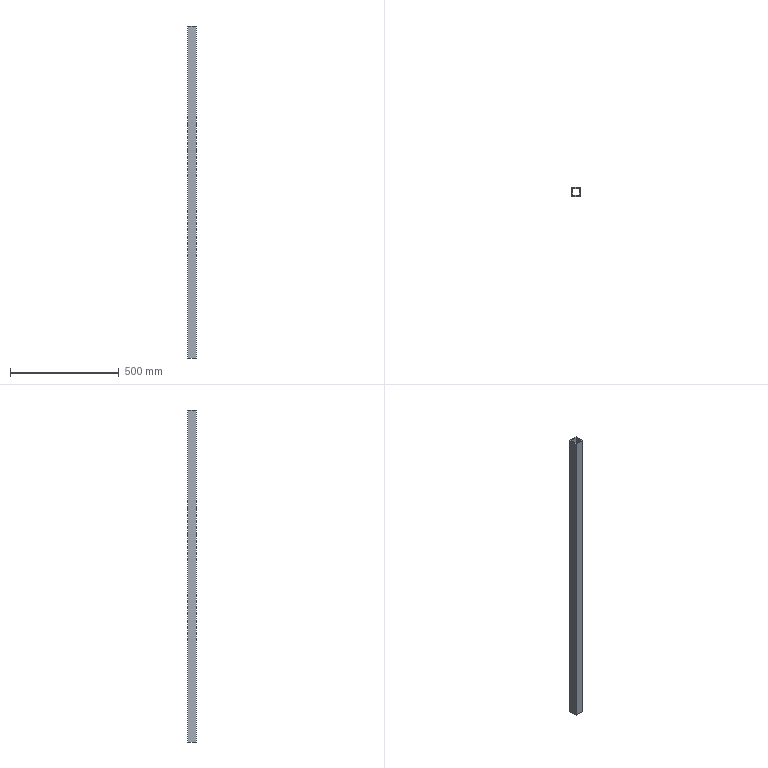Part | STEP file | ASND-0110-E63-HLTP01标准Lower机架-04 | 1 solid | 10 faces | box 40 x 40 x 1530 mm | volume 881280 mm3 | plane 10
STEP:
#1=CARTESIAN_POINT('',(0.,0.,0.));
#2=DIRECTION('',(0.,0.,1.));
#3=DIRECTION('',(1.,0.,0.));
#4=AXIS2_PLACEMENT_3D('',#1,#2,#3);
#5=CARTESIAN_POINT('',(-465.,-620.,1530.));
#6=VERTEX_POINT('',#5);
#7=CARTESIAN_POINT('',(-505.,-620.,1530.));
#8=VERTEX_POINT('',#7);
#9=CARTESIAN_POINT('',(-465.,-620.,1530.));
#10=DIRECTION('',(-1.,0.,0.));
#11=VECTOR('',#10,1.);
#12=LINE('',#9,#11);
#13=CARTESIAN_POINT('',(-505.,-620.,1586.569));
#14=DIRECTION('',(0.,-1.,0.));
#15=DIRECTION('',(0.7071,0.,0.7071));
#16=AXIS2_PLACEMENT_3D('',#13,#14,#15);
#17=PLANE('',#16);
#18=CARTESIAN_POINT('',(-11.716,-68.284));
#19=DIRECTION('',(-0.7071,0.7071));
#20=VECTOR('',#19,1.);
#21=LINE('',#18,#20);
#22=(GEOMETRIC_REPRESENTATION_CONTEXT(2)PARAMETRIC_REPRESENTATION_CONTEXT()REPRESENTATION_CONTEXT('',''));
#23=DEFINITIONAL_REPRESENTATION('',(#21),#22);
#24=PCURVE('',#17,#23);
#25=CARTESIAN_POINT('',(-60.,-1364.853,1530.));
#26=DIRECTION('',(0.,0.,1.));
#27=DIRECTION('',(0.7071,0.7071,0.));
#28=AXIS2_PLACEMENT_3D('',#25,#26,#27);
#29=PLANE('',#28);
#30=CARTESIAN_POINT('',(240.312,813.069));
#31=DIRECTION('',(-0.7071,0.7071));
#32=VECTOR('',#31,1.);
#33=LINE('',#30,#32);
#34=(GEOMETRIC_REPRESENTATION_CONTEXT(2)PARAMETRIC_REPRESENTATION_CONTEXT()REPRESENTATION_CONTEXT('',''));
#35=DEFINITIONAL_REPRESENTATION('',(#33),#34);
#36=PCURVE('',#29,#35);
#37=SURFACE_CURVE('',#12,(#24,#36),.PCURVE_S1.);
#38=EDGE_CURVE('',#6,#8,#37,.T.);
#39=ORIENTED_EDGE('',*,*,#38,.F.);
#40=CARTESIAN_POINT('',(-465.,-620.,0.));
#41=VERTEX_POINT('',#40);
#42=CARTESIAN_POINT('',(-465.,-620.,1530.));
#43=DIRECTION('',(0.,0.,-1.));
#44=VECTOR('',#43,1.);
#45=LINE('',#42,#44);
#46=CARTESIAN_POINT('',(-11.716,-68.284));
#47=DIRECTION('',(-0.7071,-0.7071));
#48=VECTOR('',#47,1.);
#49=LINE('',#46,#48);
#50=(GEOMETRIC_REPRESENTATION_CONTEXT(2)PARAMETRIC_REPRESENTATION_CONTEXT()REPRESENTATION_CONTEXT('',''));
#51=DEFINITIONAL_REPRESENTATION('',(#49),#50);
#52=PCURVE('',#17,#51);
#53=CARTESIAN_POINT('',(-465.,-660.,1586.569));
#54=DIRECTION('',(-1.,0.,0.));
#55=DIRECTION('',(0.,0.7071,0.7071));
#56=AXIS2_PLACEMENT_3D('',#53,#54,#55);
#57=PLANE('',#56);
#58=CARTESIAN_POINT('',(-11.716,68.284));
#59=DIRECTION('',(-0.7071,0.7071));
#60=VECTOR('',#59,1.);
#61=LINE('',#58,#60);
#62=(GEOMETRIC_REPRESENTATION_CONTEXT(2)PARAMETRIC_REPRESENTATION_CONTEXT()REPRESENTATION_CONTEXT('',''));
#63=DEFINITIONAL_REPRESENTATION('',(#61),#62);
#64=PCURVE('',#57,#63);
#65=SURFACE_CURVE('',#45,(#52,#64),.PCURVE_S1.);
#66=EDGE_CURVE('',#6,#41,#65,.T.);
#67=ORIENTED_EDGE('',*,*,#66,.T.);
#68=CARTESIAN_POINT('',(-505.,-620.,0.));
#69=VERTEX_POINT('',#68);
#70=CARTESIAN_POINT('',(-465.,-620.,0.));
#71=DIRECTION('',(-1.,0.,0.));
#72=VECTOR('',#71,1.);
#73=LINE('',#70,#72);
#74=CARTESIAN_POINT('',(-1093.589,-1150.158));
#75=DIRECTION('',(-0.7071,0.7071));
#76=VECTOR('',#75,1.);
#77=LINE('',#74,#76);
#78=(GEOMETRIC_REPRESENTATION_CONTEXT(2)PARAMETRIC_REPRESENTATION_CONTEXT()REPRESENTATION_CONTEXT('',''));
#79=DEFINITIONAL_REPRESENTATION('',(#77),#78);
#80=PCURVE('',#17,#79);
#81=CARTESIAN_POINT('',(0.,0.,0.));
#82=DIRECTION('',(0.,0.,-1.));
#83=DIRECTION('',(0.7071,0.7071,0.));
#84=AXIS2_PLACEMENT_3D('',#81,#82,#83);
#85=PLANE('',#84);
#86=CARTESIAN_POINT('',(-767.211,109.602));
#87=DIRECTION('',(-0.7071,-0.7071));
#88=VECTOR('',#87,1.);
#89=LINE('',#86,#88);
#90=(GEOMETRIC_REPRESENTATION_CONTEXT(2)PARAMETRIC_REPRESENTATION_CONTEXT()REPRESENTATION_CONTEXT('',''));
#91=DEFINITIONAL_REPRESENTATION('',(#89),#90);
#92=PCURVE('',#85,#91);
#93=SURFACE_CURVE('',#73,(#80,#92),.PCURVE_S1.);
#94=EDGE_CURVE('',#41,#69,#93,.T.);
#95=ORIENTED_EDGE('',*,*,#94,.T.);
#96=CARTESIAN_POINT('',(-505.,-620.,1530.));
#97=DIRECTION('',(0.,0.,-1.));
#98=VECTOR('',#97,1.);
#99=LINE('',#96,#98);
#100=CARTESIAN_POINT('',(-40.,-40.));
#101=DIRECTION('',(-0.7071,-0.7071));
#102=VECTOR('',#101,1.);
#103=LINE('',#100,#102);
#104=(GEOMETRIC_REPRESENTATION_CONTEXT(2)PARAMETRIC_REPRESENTATION_CONTEXT()REPRESENTATION_CONTEXT('',''));
#105=DEFINITIONAL_REPRESENTATION('',(#103),#104);
#106=PCURVE('',#17,#105);
#107=CARTESIAN_POINT('',(-505.,-660.,1586.569));
#108=DIRECTION('',(1.,0.,0.));
#109=DIRECTION('',(0.,0.7071,0.7071));
#110=AXIS2_PLACEMENT_3D('',#107,#108,#109);
#111=PLANE('',#110);
#112=CARTESIAN_POINT('',(-11.716,-68.284));
#113=DIRECTION('',(-0.7071,-0.7071));
#114=VECTOR('',#113,1.);
#115=LINE('',#112,#114);
#116=(GEOMETRIC_REPRESENTATION_CONTEXT(2)PARAMETRIC_REPRESENTATION_CONTEXT()REPRESENTATION_CONTEXT('',''));
#117=DEFINITIONAL_REPRESENTATION('',(#115),#116);
#118=PCURVE('',#111,#117);
#119=SURFACE_CURVE('',#99,(#106,#118),.PCURVE_S1.);
#120=EDGE_CURVE('',#8,#69,#119,.T.);
#121=ORIENTED_EDGE('',*,*,#120,.F.);
#122=EDGE_LOOP('',(#39,#67,#95,#121));
#123=FACE_BOUND('',#122,.T.);
#124=ADVANCED_FACE('',(#123),#17,.F.);
#125=CARTESIAN_POINT('',(-465.,-660.,1530.));
#126=VERTEX_POINT('',#125);
#127=CARTESIAN_POINT('',(-465.,-660.,1530.));
#128=DIRECTION('',(0.,1.,0.));
#129=VECTOR('',#128,1.);
#130=LINE('',#127,#129);
#131=CARTESIAN_POINT('',(-40.,40.));
#132=DIRECTION('',(0.7071,0.7071));
#133=VECTOR('',#132,1.);
#134=LINE('',#131,#133);
#135=(GEOMETRIC_REPRESENTATION_CONTEXT(2)PARAMETRIC_REPRESENTATION_CONTEXT()REPRESENTATION_CONTEXT('',''));
#136=DEFINITIONAL_REPRESENTATION('',(#134),#135);
#137=PCURVE('',#57,#136);
#138=CARTESIAN_POINT('',(212.028,784.784));
#139=DIRECTION('',(0.7071,0.7071));
#140=VECTOR('',#139,1.);
#141=LINE('',#138,#140);
#142=(GEOMETRIC_REPRESENTATION_CONTEXT(2)PARAMETRIC_REPRESENTATION_CONTEXT()REPRESENTATION_CONTEXT('',''));
#143=DEFINITIONAL_REPRESENTATION('',(#141),#142);
#144=PCURVE('',#29,#143);
#145=SURFACE_CURVE('',#130,(#137,#144),.PCURVE_S1.);
#146=EDGE_CURVE('',#126,#6,#145,.T.);
#147=ORIENTED_EDGE('',*,*,#146,.F.);
#148=CARTESIAN_POINT('',(-465.,-660.,0.));
#149=VERTEX_POINT('',#148);
#150=CARTESIAN_POINT('',(-465.,-660.,1530.));
#151=DIRECTION('',(0.,0.,-1.));
#152=VECTOR('',#151,1.);
#153=LINE('',#150,#152);
#154=CARTESIAN_POINT('',(-40.,40.));
#155=DIRECTION('',(-0.7071,0.7071));
#156=VECTOR('',#155,1.);
#157=LINE('',#154,#156);
#158=(GEOMETRIC_REPRESENTATION_CONTEXT(2)PARAMETRIC_REPRESENTATION_CONTEXT()REPRESENTATION_CONTEXT('',''));
#159=DEFINITIONAL_REPRESENTATION('',(#157),#158);
#160=PCURVE('',#57,#159);
#161=CARTESIAN_POINT('',(-505.,-660.,1586.569));
#162=DIRECTION('',(0.,1.,0.));
#163=DIRECTION('',(0.7071,0.,0.7071));
#164=AXIS2_PLACEMENT_3D('',#161,#162,#163);
#165=PLANE('',#164);
#166=CARTESIAN_POINT('',(-11.716,68.284));
#167=DIRECTION('',(-0.7071,0.7071));
#168=VECTOR('',#167,1.);
#169=LINE('',#166,#168);
#170=(GEOMETRIC_REPRESENTATION_CONTEXT(2)PARAMETRIC_REPRESENTATION_CONTEXT()REPRESENTATION_CONTEXT('',''));
#171=DEFINITIONAL_REPRESENTATION('',(#169),#170);
#172=PCURVE('',#165,#171);
#173=SURFACE_CURVE('',#153,(#160,#172),.PCURVE_S1.);
#174=EDGE_CURVE('',#126,#149,#173,.T.);
#175=ORIENTED_EDGE('',*,*,#174,.T.);
#176=CARTESIAN_POINT('',(-465.,-660.,0.));
#177=DIRECTION('',(0.,1.,0.));
#178=VECTOR('',#177,1.);
#179=LINE('',#176,#178);
#180=CARTESIAN_POINT('',(-1121.873,1121.873));
#181=DIRECTION('',(0.7071,0.7071));
#182=VECTOR('',#181,1.);
#183=LINE('',#180,#182);
#184=(GEOMETRIC_REPRESENTATION_CONTEXT(2)PARAMETRIC_REPRESENTATION_CONTEXT()REPRESENTATION_CONTEXT('',''));
#185=DEFINITIONAL_REPRESENTATION('',(#183),#184);
#186=PCURVE('',#57,#185);
#187=CARTESIAN_POINT('',(-795.495,137.886));
#188=DIRECTION('',(0.7071,-0.7071));
#189=VECTOR('',#188,1.);
#190=LINE('',#187,#189);
#191=(GEOMETRIC_REPRESENTATION_CONTEXT(2)PARAMETRIC_REPRESENTATION_CONTEXT()REPRESENTATION_CONTEXT('',''));
#192=DEFINITIONAL_REPRESENTATION('',(#190),#191);
#193=PCURVE('',#85,#192);
#194=SURFACE_CURVE('',#179,(#186,#193),.PCURVE_S1.);
#195=EDGE_CURVE('',#149,#41,#194,.T.);
#196=ORIENTED_EDGE('',*,*,#195,.T.);
#197=ORIENTED_EDGE('',*,*,#66,.F.);
#198=EDGE_LOOP('',(#147,#175,#196,#197));
#199=FACE_BOUND('',#198,.T.);
#200=ADVANCED_FACE('',(#199),#57,.F.);
#201=CARTESIAN_POINT('',(-505.,-660.,1530.));
#202=VERTEX_POINT('',#201);
#203=CARTESIAN_POINT('',(-505.,-660.,1530.));
#204=DIRECTION('',(1.,0.,0.));
#205=VECTOR('',#204,1.);
#206=LINE('',#203,#205);
#207=CARTESIAN_POINT('',(-40.,40.));
#208=DIRECTION('',(0.7071,0.7071));
#209=VECTOR('',#208,1.);
#210=LINE('',#207,#209);
#211=(GEOMETRIC_REPRESENTATION_CONTEXT(2)PARAMETRIC_REPRESENTATION_CONTEXT()REPRESENTATION_CONTEXT('',''));
#212=DEFINITIONAL_REPRESENTATION('',(#210),#211);
#213=PCURVE('',#165,#212);
#214=CARTESIAN_POINT('',(183.744,813.069));
#215=DIRECTION('',(0.7071,-0.7071));
#216=VECTOR('',#215,1.);
#217=LINE('',#214,#216);
#218=(GEOMETRIC_REPRESENTATION_CONTEXT(2)PARAMETRIC_REPRESENTATION_CONTEXT()REPRESENTATION_CONTEXT('',''));
#219=DEFINITIONAL_REPRESENTATION('',(#217),#218);
#220=PCURVE('',#29,#219);
#221=SURFACE_CURVE('',#206,(#213,#220),.PCURVE_S1.);
#222=EDGE_CURVE('',#202,#126,#221,.T.);
#223=ORIENTED_EDGE('',*,*,#222,.F.);
#224=CARTESIAN_POINT('',(-505.,-660.,0.));
#225=VERTEX_POINT('',#224);
#226=CARTESIAN_POINT('',(-505.,-660.,1530.));
#227=DIRECTION('',(0.,0.,-1.));
#228=VECTOR('',#227,1.);
#229=LINE('',#226,#228);
#230=CARTESIAN_POINT('',(-40.,40.));
#231=DIRECTION('',(-0.7071,0.7071));
#232=VECTOR('',#231,1.);
#233=LINE('',#230,#232);
#234=(GEOMETRIC_REPRESENTATION_CONTEXT(2)PARAMETRIC_REPRESENTATION_CONTEXT()REPRESENTATION_CONTEXT('',''));
#235=DEFINITIONAL_REPRESENTATION('',(#233),#234);
#236=PCURVE('',#165,#235);
#237=CARTESIAN_POINT('',(-40.,-40.));
#238=DIRECTION('',(-0.7071,-0.7071));
#239=VECTOR('',#238,1.);
#240=LINE('',#237,#239);
#241=(GEOMETRIC_REPRESENTATION_CONTEXT(2)PARAMETRIC_REPRESENTATION_CONTEXT()REPRESENTATION_CONTEXT('',''));
#242=DEFINITIONAL_REPRESENTATION('',(#240),#241);
#243=PCURVE('',#111,#242);
#244=SURFACE_CURVE('',#229,(#236,#243),.PCURVE_S1.);
#245=EDGE_CURVE('',#202,#225,#244,.T.);
#246=ORIENTED_EDGE('',*,*,#245,.T.);
#247=CARTESIAN_POINT('',(-505.,-660.,0.));
#248=DIRECTION('',(1.,0.,0.));
#249=VECTOR('',#248,1.);
#250=LINE('',#247,#249);
#251=CARTESIAN_POINT('',(-1121.873,1121.873));
#252=DIRECTION('',(0.7071,0.7071));
#253=VECTOR('',#252,1.);
#254=LINE('',#251,#253);
#255=(GEOMETRIC_REPRESENTATION_CONTEXT(2)PARAMETRIC_REPRESENTATION_CONTEXT()REPRESENTATION_CONTEXT('',''));
#256=DEFINITIONAL_REPRESENTATION('',(#254),#255);
#257=PCURVE('',#165,#256);
#258=CARTESIAN_POINT('',(-823.779,109.602));
#259=DIRECTION('',(0.7071,0.7071));
#260=VECTOR('',#259,1.);
#261=LINE('',#258,#260);
#262=(GEOMETRIC_REPRESENTATION_CONTEXT(2)PARAMETRIC_REPRESENTATION_CONTEXT()REPRESENTATION_CONTEXT('',''));
#263=DEFINITIONAL_REPRESENTATION('',(#261),#262);
#264=PCURVE('',#85,#263);
#265=SURFACE_CURVE('',#250,(#257,#264),.PCURVE_S1.);
#266=EDGE_CURVE('',#225,#149,#265,.T.);
#267=ORIENTED_EDGE('',*,*,#266,.T.);
#268=ORIENTED_EDGE('',*,*,#174,.F.);
#269=EDGE_LOOP('',(#223,#246,#267,#268));
#270=FACE_BOUND('',#269,.T.);
#271=ADVANCED_FACE('',(#270),#165,.F.);
#272=CARTESIAN_POINT('',(-505.,-620.,1530.));
#273=DIRECTION('',(0.,-1.,0.));
#274=VECTOR('',#273,1.);
#275=LINE('',#272,#274);
#276=CARTESIAN_POINT('',(-11.716,-68.284));
#277=DIRECTION('',(-0.7071,0.7071));
#278=VECTOR('',#277,1.);
#279=LINE('',#276,#278);
#280=(GEOMETRIC_REPRESENTATION_CONTEXT(2)PARAMETRIC_REPRESENTATION_CONTEXT()REPRESENTATION_CONTEXT('',''));
#281=DEFINITIONAL_REPRESENTATION('',(#279),#280);
#282=PCURVE('',#111,#281);
#283=CARTESIAN_POINT('',(212.028,841.353));
#284=DIRECTION('',(-0.7071,-0.7071));
#285=VECTOR('',#284,1.);
#286=LINE('',#283,#285);
#287=(GEOMETRIC_REPRESENTATION_CONTEXT(2)PARAMETRIC_REPRESENTATION_CONTEXT()REPRESENTATION_CONTEXT('',''));
#288=DEFINITIONAL_REPRESENTATION('',(#286),#287);
#289=PCURVE('',#29,#288);
#290=SURFACE_CURVE('',#275,(#282,#289),.PCURVE_S1.);
#291=EDGE_CURVE('',#8,#202,#290,.T.);
#292=ORIENTED_EDGE('',*,*,#291,.F.);
#293=ORIENTED_EDGE('',*,*,#120,.T.);
#294=CARTESIAN_POINT('',(-505.,-620.,0.));
#295=DIRECTION('',(0.,-1.,0.));
#296=VECTOR('',#295,1.);
#297=LINE('',#294,#296);
#298=CARTESIAN_POINT('',(-1093.589,-1150.158));
#299=DIRECTION('',(-0.7071,0.7071));
#300=VECTOR('',#299,1.);
#301=LINE('',#298,#300);
#302=(GEOMETRIC_REPRESENTATION_CONTEXT(2)PARAMETRIC_REPRESENTATION_CONTEXT()REPRESENTATION_CONTEXT('',''));
#303=DEFINITIONAL_REPRESENTATION('',(#301),#302);
#304=PCURVE('',#111,#303);
#305=CARTESIAN_POINT('',(-795.495,81.317));
#306=DIRECTION('',(-0.7071,0.7071));
#307=VECTOR('',#306,1.);
#308=LINE('',#305,#307);
#309=(GEOMETRIC_REPRESENTATION_CONTEXT(2)PARAMETRIC_REPRESENTATION_CONTEXT()REPRESENTATION_CONTEXT('',''));
#310=DEFINITIONAL_REPRESENTATION('',(#308),#309);
#311=PCURVE('',#85,#310);
#312=SURFACE_CURVE('',#297,(#304,#311),.PCURVE_S1.);
#313=EDGE_CURVE('',#69,#225,#312,.T.);
#314=ORIENTED_EDGE('',*,*,#313,.T.);
#315=ORIENTED_EDGE('',*,*,#245,.F.);
#316=EDGE_LOOP('',(#292,#293,#314,#315));
#317=FACE_BOUND('',#316,.T.);
#318=ADVANCED_FACE('',(#317),#111,.F.);
#319=ORIENTED_EDGE('',*,*,#313,.F.);
#320=ORIENTED_EDGE('',*,*,#94,.F.);
#321=ORIENTED_EDGE('',*,*,#195,.F.);
#322=ORIENTED_EDGE('',*,*,#266,.F.);
#323=EDGE_LOOP('',(#319,#320,#321,#322));
#324=FACE_BOUND('',#323,.T.);
#325=CARTESIAN_POINT('',(-469.,-624.,0.));
#326=VERTEX_POINT('',#325);
#327=CARTESIAN_POINT('',(-501.,-624.,0.));
#328=VERTEX_POINT('',#327);
#329=CARTESIAN_POINT('',(-469.,-624.,0.));
#330=DIRECTION('',(-1.,0.,0.));
#331=VECTOR('',#330,1.);
#332=LINE('',#329,#331);
#333=CARTESIAN_POINT('',(-772.868,109.602));
#334=DIRECTION('',(-0.7071,-0.7071));
#335=VECTOR('',#334,1.);
#336=LINE('',#333,#335);
#337=(GEOMETRIC_REPRESENTATION_CONTEXT(2)PARAMETRIC_REPRESENTATION_CONTEXT()REPRESENTATION_CONTEXT('',''));
#338=DEFINITIONAL_REPRESENTATION('',(#336),#337);
#339=PCURVE('',#85,#338);
#340=CARTESIAN_POINT('',(-501.,-624.,1586.569));
#341=DIRECTION('',(0.,-1.,0.));
#342=DIRECTION('',(0.7071,0.,0.7071));
#343=AXIS2_PLACEMENT_3D('',#340,#341,#342);
#344=PLANE('',#343);
#345=CARTESIAN_POINT('',(-1099.246,-1144.501));
#346=DIRECTION('',(-0.7071,0.7071));
#347=VECTOR('',#346,1.);
#348=LINE('',#345,#347);
#349=(GEOMETRIC_REPRESENTATION_CONTEXT(2)PARAMETRIC_REPRESENTATION_CONTEXT()REPRESENTATION_CONTEXT('',''));
#350=DEFINITIONAL_REPRESENTATION('',(#348),#349);
#351=PCURVE('',#344,#350);
#352=SURFACE_CURVE('',#332,(#339,#351),.PCURVE_S1.);
#353=EDGE_CURVE('',#326,#328,#352,.T.);
#354=ORIENTED_EDGE('',*,*,#353,.T.);
#355=CARTESIAN_POINT('',(-501.,-656.,0.));
#356=VERTEX_POINT('',#355);
#357=CARTESIAN_POINT('',(-501.,-624.,0.));
#358=DIRECTION('',(0.,-1.,0.));
#359=VECTOR('',#358,1.);
#360=LINE('',#357,#359);
#361=CARTESIAN_POINT('',(-795.495,86.974));
#362=DIRECTION('',(-0.7071,0.7071));
#363=VECTOR('',#362,1.);
#364=LINE('',#361,#363);
#365=(GEOMETRIC_REPRESENTATION_CONTEXT(2)PARAMETRIC_REPRESENTATION_CONTEXT()REPRESENTATION_CONTEXT('',''));
#366=DEFINITIONAL_REPRESENTATION('',(#364),#365);
#367=PCURVE('',#85,#366);
#368=CARTESIAN_POINT('',(-501.,-656.,1586.569));
#369=DIRECTION('',(1.,0.,0.));
#370=DIRECTION('',(0.,0.7071,0.7071));
#371=AXIS2_PLACEMENT_3D('',#368,#369,#370);
#372=PLANE('',#371);
#373=CARTESIAN_POINT('',(-1099.246,-1144.501));
#374=DIRECTION('',(-0.7071,0.7071));
#375=VECTOR('',#374,1.);
#376=LINE('',#373,#375);
#377=(GEOMETRIC_REPRESENTATION_CONTEXT(2)PARAMETRIC_REPRESENTATION_CONTEXT()REPRESENTATION_CONTEXT('',''));
#378=DEFINITIONAL_REPRESENTATION('',(#376),#377);
#379=PCURVE('',#372,#378);
#380=SURFACE_CURVE('',#360,(#367,#379),.PCURVE_S1.);
#381=EDGE_CURVE('',#328,#356,#380,.T.);
#382=ORIENTED_EDGE('',*,*,#381,.T.);
#383=CARTESIAN_POINT('',(-469.,-656.,0.));
#384=VERTEX_POINT('',#383);
#385=CARTESIAN_POINT('',(-501.,-656.,0.));
#386=DIRECTION('',(1.,0.,0.));
#387=VECTOR('',#386,1.);
#388=LINE('',#385,#387);
#389=CARTESIAN_POINT('',(-818.123,109.602));
#390=DIRECTION('',(0.7071,0.7071));
#391=VECTOR('',#390,1.);
#392=LINE('',#389,#391);
#393=(GEOMETRIC_REPRESENTATION_CONTEXT(2)PARAMETRIC_REPRESENTATION_CONTEXT()REPRESENTATION_CONTEXT('',''));
#394=DEFINITIONAL_REPRESENTATION('',(#392),#393);
#395=PCURVE('',#85,#394);
#396=CARTESIAN_POINT('',(-501.,-656.,1586.569));
#397=DIRECTION('',(0.,1.,0.));
#398=DIRECTION('',(0.7071,0.,0.7071));
#399=AXIS2_PLACEMENT_3D('',#396,#397,#398);
#400=PLANE('',#399);
#401=CARTESIAN_POINT('',(-1121.873,1121.873));
#402=DIRECTION('',(0.7071,0.7071));
#403=VECTOR('',#402,1.);
#404=LINE('',#401,#403);
#405=(GEOMETRIC_REPRESENTATION_CONTEXT(2)PARAMETRIC_REPRESENTATION_CONTEXT()REPRESENTATION_CONTEXT('',''));
#406=DEFINITIONAL_REPRESENTATION('',(#404),#405);
#407=PCURVE('',#400,#406);
#408=SURFACE_CURVE('',#388,(#395,#407),.PCURVE_S1.);
#409=EDGE_CURVE('',#356,#384,#408,.T.);
#410=ORIENTED_EDGE('',*,*,#409,.T.);
#411=CARTESIAN_POINT('',(-469.,-656.,0.));
#412=DIRECTION('',(0.,1.,0.));
#413=VECTOR('',#412,1.);
#414=LINE('',#411,#413);
#415=CARTESIAN_POINT('',(-795.495,132.229));
#416=DIRECTION('',(0.7071,-0.7071));
#417=VECTOR('',#416,1.);
#418=LINE('',#415,#417);
#419=(GEOMETRIC_REPRESENTATION_CONTEXT(2)PARAMETRIC_REPRESENTATION_CONTEXT()REPRESENTATION_CONTEXT('',''));
#420=DEFINITIONAL_REPRESENTATION('',(#418),#419);
#421=PCURVE('',#85,#420);
#422=CARTESIAN_POINT('',(-469.,-656.,1586.569));
#423=DIRECTION('',(-1.,0.,0.));
#424=DIRECTION('',(0.,0.7071,0.7071));
#425=AXIS2_PLACEMENT_3D('',#422,#423,#424);
#426=PLANE('',#425);
#427=CARTESIAN_POINT('',(-1121.873,1121.873));
#428=DIRECTION('',(0.7071,0.7071));
#429=VECTOR('',#428,1.);
#430=LINE('',#427,#429);
#431=(GEOMETRIC_REPRESENTATION_CONTEXT(2)PARAMETRIC_REPRESENTATION_CONTEXT()REPRESENTATION_CONTEXT('',''));
#432=DEFINITIONAL_REPRESENTATION('',(#430),#431);
#433=PCURVE('',#426,#432);
#434=SURFACE_CURVE('',#414,(#421,#433),.PCURVE_S1.);
#435=EDGE_CURVE('',#384,#326,#434,.T.);
#436=ORIENTED_EDGE('',*,*,#435,.T.);
#437=EDGE_LOOP('',(#354,#382,#410,#436));
#438=FACE_BOUND('',#437,.T.);
#439=ADVANCED_FACE('',(#324,#438),#85,.T.);
#440=CARTESIAN_POINT('',(-469.,-624.,1530.));
#441=VERTEX_POINT('',#440);
#442=CARTESIAN_POINT('',(-469.,-624.,1530.));
#443=DIRECTION('',(0.,0.,-1.));
#444=VECTOR('',#443,1.);
#445=LINE('',#442,#444);
#446=CARTESIAN_POINT('',(-17.373,-62.627));
#447=DIRECTION('',(-0.7071,-0.7071));
#448=VECTOR('',#447,1.);
#449=LINE('',#446,#448);
#450=(GEOMETRIC_REPRESENTATION_CONTEXT(2)PARAMETRIC_REPRESENTATION_CONTEXT()REPRESENTATION_CONTEXT('',''));
#451=DEFINITIONAL_REPRESENTATION('',(#449),#450);
#452=PCURVE('',#344,#451);
#453=CARTESIAN_POINT('',(-17.373,62.627));
#454=DIRECTION('',(-0.7071,0.7071));
#455=VECTOR('',#454,1.);
#456=LINE('',#453,#455);
#457=(GEOMETRIC_REPRESENTATION_CONTEXT(2)PARAMETRIC_REPRESENTATION_CONTEXT()REPRESENTATION_CONTEXT('',''));
#458=DEFINITIONAL_REPRESENTATION('',(#456),#457);
#459=PCURVE('',#426,#458);
#460=SURFACE_CURVE('',#445,(#452,#459),.PCURVE_S1.);
#461=EDGE_CURVE('',#441,#326,#460,.T.);
#462=ORIENTED_EDGE('',*,*,#461,.F.);
#463=CARTESIAN_POINT('',(-501.,-624.,1530.));
#464=VERTEX_POINT('',#463);
#465=CARTESIAN_POINT('',(-469.,-624.,1530.));
#466=DIRECTION('',(-1.,0.,0.));
#467=VECTOR('',#466,1.);
#468=LINE('',#465,#467);
#469=CARTESIAN_POINT('',(-17.373,-62.627));
#470=DIRECTION('',(-0.7071,0.7071));
#471=VECTOR('',#470,1.);
#472=LINE('',#469,#471);
#473=(GEOMETRIC_REPRESENTATION_CONTEXT(2)PARAMETRIC_REPRESENTATION_CONTEXT()REPRESENTATION_CONTEXT('',''));
#474=DEFINITIONAL_REPRESENTATION('',(#472),#473);
#475=PCURVE('',#344,#474);
#476=CARTESIAN_POINT('',(234.655,813.069));
#477=DIRECTION('',(-0.7071,0.7071));
#478=VECTOR('',#477,1.);
#479=LINE('',#476,#478);
#480=(GEOMETRIC_REPRESENTATION_CONTEXT(2)PARAMETRIC_REPRESENTATION_CONTEXT()REPRESENTATION_CONTEXT('',''));
#481=DEFINITIONAL_REPRESENTATION('',(#479),#480);
#482=PCURVE('',#29,#481);
#483=SURFACE_CURVE('',#468,(#475,#482),.PCURVE_S1.);
#484=EDGE_CURVE('',#441,#464,#483,.T.);
#485=ORIENTED_EDGE('',*,*,#484,.T.);
#486=CARTESIAN_POINT('',(-501.,-624.,1530.));
#487=DIRECTION('',(0.,0.,-1.));
#488=VECTOR('',#487,1.);
#489=LINE('',#486,#488);
#490=CARTESIAN_POINT('',(-40.,-40.));
#491=DIRECTION('',(-0.7071,-0.7071));
#492=VECTOR('',#491,1.);
#493=LINE('',#490,#492);
#494=(GEOMETRIC_REPRESENTATION_CONTEXT(2)PARAMETRIC_REPRESENTATION_CONTEXT()REPRESENTATION_CONTEXT('',''));
#495=DEFINITIONAL_REPRESENTATION('',(#493),#494);
#496=PCURVE('',#344,#495);
#497=CARTESIAN_POINT('',(-17.373,-62.627));
#498=DIRECTION('',(-0.7071,-0.7071));
#499=VECTOR('',#498,1.);
#500=LINE('',#497,#499);
#501=(GEOMETRIC_REPRESENTATION_CONTEXT(2)PARAMETRIC_REPRESENTATION_CONTEXT()REPRESENTATION_CONTEXT('',''));
#502=DEFINITIONAL_REPRESENTATION('',(#500),#501);
#503=PCURVE('',#372,#502);
#504=SURFACE_CURVE('',#489,(#496,#503),.PCURVE_S1.);
#505=EDGE_CURVE('',#464,#328,#504,.T.);
#506=ORIENTED_EDGE('',*,*,#505,.T.);
#507=ORIENTED_EDGE('',*,*,#353,.F.);
#508=EDGE_LOOP('',(#462,#485,#506,#507));
#509=FACE_BOUND('',#508,.T.);
#510=ADVANCED_FACE('',(#509),#344,.T.);
#511=CARTESIAN_POINT('',(-469.,-656.,1530.));
#512=VERTEX_POINT('',#511);
#513=CARTESIAN_POINT('',(-469.,-656.,1530.));
#514=DIRECTION('',(0.,0.,-1.));
#515=VECTOR('',#514,1.);
#516=LINE('',#513,#515);
#517=CARTESIAN_POINT('',(-40.,40.));
#518=DIRECTION('',(-0.7071,0.7071));
#519=VECTOR('',#518,1.);
#520=LINE('',#517,#519);
#521=(GEOMETRIC_REPRESENTATION_CONTEXT(2)PARAMETRIC_REPRESENTATION_CONTEXT()REPRESENTATION_CONTEXT('',''));
#522=DEFINITIONAL_REPRESENTATION('',(#520),#521);
#523=PCURVE('',#426,#522);
#524=CARTESIAN_POINT('',(-17.373,62.627));
#525=DIRECTION('',(-0.7071,0.7071));
#526=VECTOR('',#525,1.);
#527=LINE('',#524,#526);
#528=(GEOMETRIC_REPRESENTATION_CONTEXT(2)PARAMETRIC_REPRESENTATION_CONTEXT()REPRESENTATION_CONTEXT('',''));
#529=DEFINITIONAL_REPRESENTATION('',(#527),#528);
#530=PCURVE('',#400,#529);
#531=SURFACE_CURVE('',#516,(#523,#530),.PCURVE_S1.);
#532=EDGE_CURVE('',#512,#384,#531,.T.);
#533=ORIENTED_EDGE('',*,*,#532,.F.);
#534=CARTESIAN_POINT('',(-469.,-656.,1530.));
#535=DIRECTION('',(0.,1.,0.));
#536=VECTOR('',#535,1.);
#537=LINE('',#534,#536);
#538=CARTESIAN_POINT('',(-40.,40.));
#539=DIRECTION('',(0.7071,0.7071));
#540=VECTOR('',#539,1.);
#541=LINE('',#538,#540);
#542=(GEOMETRIC_REPRESENTATION_CONTEXT(2)PARAMETRIC_REPRESENTATION_CONTEXT()REPRESENTATION_CONTEXT('',''));
#543=DEFINITIONAL_REPRESENTATION('',(#541),#542);
#544=PCURVE('',#426,#543);
#545=CARTESIAN_POINT('',(212.028,790.441));
#546=DIRECTION('',(0.7071,0.7071));
#547=VECTOR('',#546,1.);
#548=LINE('',#545,#547);
#549=(GEOMETRIC_REPRESENTATION_CONTEXT(2)PARAMETRIC_REPRESENTATION_CONTEXT()REPRESENTATION_CONTEXT('',''));
#550=DEFINITIONAL_REPRESENTATION('',(#548),#549);
#551=PCURVE('',#29,#550);
#552=SURFACE_CURVE('',#537,(#544,#551),.PCURVE_S1.);
#553=EDGE_CURVE('',#512,#441,#552,.T.);
#554=ORIENTED_EDGE('',*,*,#553,.T.);
#555=ORIENTED_EDGE('',*,*,#461,.T.);
#556=ORIENTED_EDGE('',*,*,#435,.F.);
#557=EDGE_LOOP('',(#533,#554,#555,#556));
#558=FACE_BOUND('',#557,.T.);
#559=ADVANCED_FACE('',(#558),#426,.T.);
#560=CARTESIAN_POINT('',(-501.,-656.,1530.));
#561=VERTEX_POINT('',#560);
#562=CARTESIAN_POINT('',(-501.,-656.,1530.));
#563=DIRECTION('',(0.,0.,-1.));
#564=VECTOR('',#563,1.);
#565=LINE('',#562,#564);
#566=CARTESIAN_POINT('',(-40.,40.));
#567=DIRECTION('',(-0.7071,0.7071));
#568=VECTOR('',#567,1.);
#569=LINE('',#566,#568);
#570=(GEOMETRIC_REPRESENTATION_CONTEXT(2)PARAMETRIC_REPRESENTATION_CONTEXT()REPRESENTATION_CONTEXT('',''));
#571=DEFINITIONAL_REPRESENTATION('',(#569),#570);
#572=PCURVE('',#400,#571);
#573=CARTESIAN_POINT('',(-40.,-40.));
#574=DIRECTION('',(-0.7071,-0.7071));
#575=VECTOR('',#574,1.);
#576=LINE('',#573,#575);
#577=(GEOMETRIC_REPRESENTATION_CONTEXT(2)PARAMETRIC_REPRESENTATION_CONTEXT()REPRESENTATION_CONTEXT('',''));
#578=DEFINITIONAL_REPRESENTATION('',(#576),#577);
#579=PCURVE('',#372,#578);
#580=SURFACE_CURVE('',#565,(#572,#579),.PCURVE_S1.);
#581=EDGE_CURVE('',#561,#356,#580,.T.);
#582=ORIENTED_EDGE('',*,*,#581,.F.);
#583=CARTESIAN_POINT('',(-501.,-656.,1530.));
#584=DIRECTION('',(1.,0.,0.));
#585=VECTOR('',#584,1.);
#586=LINE('',#583,#585);
#587=CARTESIAN_POINT('',(-40.,40.));
#588=DIRECTION('',(0.7071,0.7071));
#589=VECTOR('',#588,1.);
#590=LINE('',#587,#589);
#591=(GEOMETRIC_REPRESENTATION_CONTEXT(2)PARAMETRIC_REPRESENTATION_CONTEXT()REPRESENTATION_CONTEXT('',''));
#592=DEFINITIONAL_REPRESENTATION('',(#590),#591);
#593=PCURVE('',#400,#592);
#594=CARTESIAN_POINT('',(189.401,813.069));
#595=DIRECTION('',(0.7071,-0.7071));
#596=VECTOR('',#595,1.);
#597=LINE('',#594,#596);
#598=(GEOMETRIC_REPRESENTATION_CONTEXT(2)PARAMETRIC_REPRESENTATION_CONTEXT()REPRESENTATION_CONTEXT('',''));
#599=DEFINITIONAL_REPRESENTATION('',(#597),#598);
#600=PCURVE('',#29,#599);
#601=SURFACE_CURVE('',#586,(#593,#600),.PCURVE_S1.);
#602=EDGE_CURVE('',#561,#512,#601,.T.);
#603=ORIENTED_EDGE('',*,*,#602,.T.);
#604=ORIENTED_EDGE('',*,*,#532,.T.);
#605=ORIENTED_EDGE('',*,*,#409,.F.);
#606=EDGE_LOOP('',(#582,#603,#604,#605));
#607=FACE_BOUND('',#606,.T.);
#608=ADVANCED_FACE('',(#607),#400,.T.);
#609=ORIENTED_EDGE('',*,*,#505,.F.);
#610=CARTESIAN_POINT('',(-501.,-624.,1530.));
#611=DIRECTION('',(0.,-1.,0.));
#612=VECTOR('',#611,1.);
#613=LINE('',#610,#612);
#614=CARTESIAN_POINT('',(-17.373,-62.627));
#615=DIRECTION('',(-0.7071,0.7071));
#616=VECTOR('',#615,1.);
#617=LINE('',#614,#616);
#618=(GEOMETRIC_REPRESENTATION_CONTEXT(2)PARAMETRIC_REPRESENTATION_CONTEXT()REPRESENTATION_CONTEXT('',''));
#619=DEFINITIONAL_REPRESENTATION('',(#617),#618);
#620=PCURVE('',#372,#619);
#621=CARTESIAN_POINT('',(212.028,835.696));
#622=DIRECTION('',(-0.7071,-0.7071));
#623=VECTOR('',#622,1.);
#624=LINE('',#621,#623);
#625=(GEOMETRIC_REPRESENTATION_CONTEXT(2)PARAMETRIC_REPRESENTATION_CONTEXT()REPRESENTATION_CONTEXT('',''));
#626=DEFINITIONAL_REPRESENTATION('',(#624),#625);
#627=PCURVE('',#29,#626);
#628=SURFACE_CURVE('',#613,(#620,#627),.PCURVE_S1.);
#629=EDGE_CURVE('',#464,#561,#628,.T.);
#630=ORIENTED_EDGE('',*,*,#629,.T.);
#631=ORIENTED_EDGE('',*,*,#581,.T.);
#632=ORIENTED_EDGE('',*,*,#381,.F.);
#633=EDGE_LOOP('',(#609,#630,#631,#632));
#634=FACE_BOUND('',#633,.T.);
#635=ADVANCED_FACE('',(#634),#372,.T.);
#636=ORIENTED_EDGE('',*,*,#38,.T.);
#637=ORIENTED_EDGE('',*,*,#291,.T.);
#638=ORIENTED_EDGE('',*,*,#222,.T.);
#639=ORIENTED_EDGE('',*,*,#146,.T.);
#640=EDGE_LOOP('',(#636,#637,#638,#639));
#641=FACE_BOUND('',#640,.T.);
#642=ORIENTED_EDGE('',*,*,#629,.F.);
#643=ORIENTED_EDGE('',*,*,#484,.F.);
#644=ORIENTED_EDGE('',*,*,#553,.F.);
#645=ORIENTED_EDGE('',*,*,#602,.F.);
#646=EDGE_LOOP('',(#642,#643,#644,#645));
#647=FACE_BOUND('',#646,.T.);
#648=ADVANCED_FACE('',(#641,#647),#29,.T.);
#649=CLOSED_SHELL('',(#124,#200,#271,#318,#439,#510,#559,#608,#635,#648));
#650=MANIFOLD_SOLID_BREP('',#649);
#651=(LENGTH_UNIT()NAMED_UNIT(*)SI_UNIT(.MILLI.,.METRE.));
#652=UNCERTAINTY_MEASURE_WITH_UNIT(LENGTH_MEASURE(0.0000001),#651,'','');
#653=(NAMED_UNIT(*)PLANE_ANGLE_UNIT()SI_UNIT($,.RADIAN.));
#654=(NAMED_UNIT(*)SI_UNIT($,.STERADIAN.)SOLID_ANGLE_UNIT());
#655=(GEOMETRIC_REPRESENTATION_CONTEXT(3)GLOBAL_UNCERTAINTY_ASSIGNED_CONTEXT((#652))GLOBAL_UNIT_ASSIGNED_CONTEXT((#651,#653,#654))REPRESENTATION_CONTEXT('',''));
#656=ADVANCED_BREP_SHAPE_REPRESENTATION('',(#4,#650),#655);